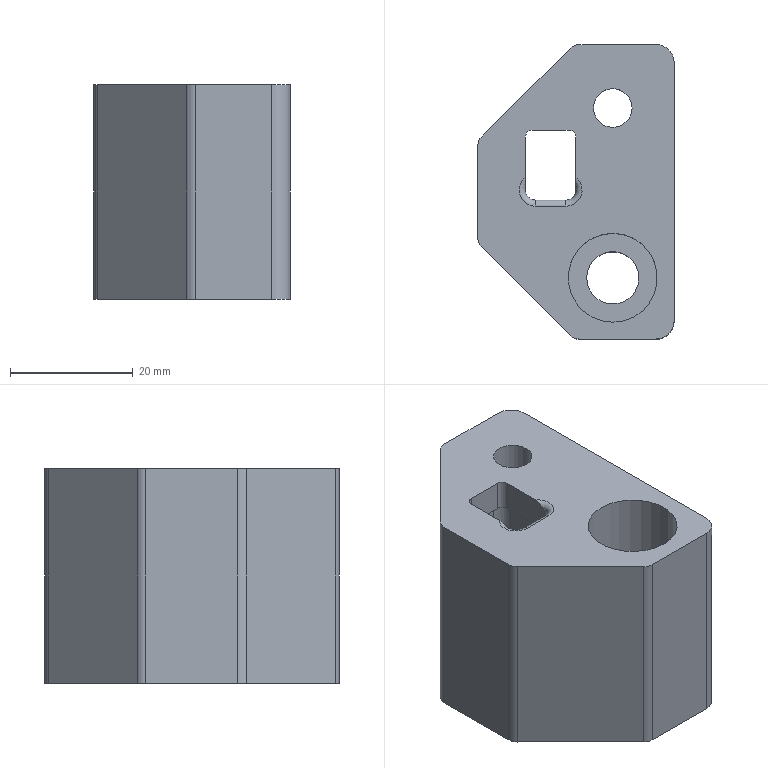Part | NX | features DIE-14 2 | 1 solid | 39 faces | box 32 x 48 x 35 mm | volume 36038 mm3 | cylinder 19 | plane 18 | torus 2 | commonest cylinder face diameters 4 x6 2.24 x2 3.24 x2 5 x2 6 x2 2 x1
STEP:
#1=CARTESIAN_POINT('',(2411.699,-953.548,823.716));
#2=VERTEX_POINT('',#1);
#3=CARTESIAN_POINT('',(2411.699,-911.548,823.716));
#4=VERTEX_POINT('',#3);
#5=CARTESIAN_POINT('',(2411.699,-928.548,823.716));
#6=DIRECTION('',(0.,1.,0.));
#7=VECTOR('',#6,1000.);
#8=LINE('',#5,#7);
#9=EDGE_CURVE('',#2,#4,#8,.T.);
#10=ORIENTED_EDGE('',*,*,#9,.T.);
#11=CARTESIAN_POINT('',(2411.699,-911.548,858.716));
#12=VERTEX_POINT('',#11);
#13=CARTESIAN_POINT('',(2411.699,-911.548,858.716));
#14=DIRECTION('',(0.,0.,1.));
#15=VECTOR('',#14,1000.);
#16=LINE('',#13,#15);
#17=EDGE_CURVE('',#4,#12,#16,.T.);
#18=ORIENTED_EDGE('',*,*,#17,.T.);
#19=CARTESIAN_POINT('',(2411.699,-953.548,858.716));
#20=VERTEX_POINT('',#19);
#21=CARTESIAN_POINT('',(2411.699,-928.548,858.716));
#22=DIRECTION('',(0.,-1.,0.));
#23=VECTOR('',#22,1000.);
#24=LINE('',#21,#23);
#25=EDGE_CURVE('',#12,#20,#24,.T.);
#26=ORIENTED_EDGE('',*,*,#25,.T.);
#27=CARTESIAN_POINT('',(2411.699,-953.548,858.716));
#28=DIRECTION('',(0.,0.,1.));
#29=VECTOR('',#28,1000.);
#30=LINE('',#27,#29);
#31=EDGE_CURVE('',#20,#2,#30,.F.);
#32=ORIENTED_EDGE('',*,*,#31,.T.);
#33=EDGE_LOOP('',(#10,#18,#26,#32));
#34=FACE_BOUND('',#33,.T.);
#35=CARTESIAN_POINT('',(2411.699,-928.548,858.716));
#36=DIRECTION('',(1.,0.,0.));
#37=DIRECTION('',(0.,0.,1.));
#38=AXIS2_PLACEMENT_3D('',#35,#36,#37);
#39=PLANE('',#38);
#40=ADVANCED_FACE('',(#34),#39,.T.);
#41=CARTESIAN_POINT('',(2396.185,-908.548,858.716));
#42=VERTEX_POINT('',#41);
#43=CARTESIAN_POINT('',(2408.699,-908.548,858.716));
#44=VERTEX_POINT('',#43);
#45=CARTESIAN_POINT('',(2401.699,-908.548,858.716));
#46=DIRECTION('',(1.,0.,0.));
#47=VECTOR('',#46,1000.);
#48=LINE('',#45,#47);
#49=EDGE_CURVE('',#42,#44,#48,.T.);
#50=ORIENTED_EDGE('',*,*,#49,.T.);
#51=CARTESIAN_POINT('',(2408.699,-908.548,823.716));
#52=VERTEX_POINT('',#51);
#53=CARTESIAN_POINT('',(2408.699,-908.548,858.716));
#54=DIRECTION('',(0.,0.,1.));
#55=VECTOR('',#54,1000.);
#56=LINE('',#53,#55);
#57=EDGE_CURVE('',#44,#52,#56,.F.);
#58=ORIENTED_EDGE('',*,*,#57,.T.);
#59=CARTESIAN_POINT('',(2396.185,-908.548,823.716));
#60=VERTEX_POINT('',#59);
#61=CARTESIAN_POINT('',(2401.699,-908.548,823.716));
#62=DIRECTION('',(-1.,0.,0.));
#63=VECTOR('',#62,1000.);
#64=LINE('',#61,#63);
#65=EDGE_CURVE('',#52,#60,#64,.T.);
#66=ORIENTED_EDGE('',*,*,#65,.T.);
#67=CARTESIAN_POINT('',(2396.185,-908.548,858.716));
#68=DIRECTION('',(0.,0.,-1.));
#69=VECTOR('',#68,1000.);
#70=LINE('',#67,#69);
#71=EDGE_CURVE('',#60,#42,#70,.F.);
#72=ORIENTED_EDGE('',*,*,#71,.T.);
#73=EDGE_LOOP('',(#50,#58,#66,#72));
#74=FACE_BOUND('',#73,.T.);
#75=CARTESIAN_POINT('',(2401.699,-908.548,858.716));
#76=DIRECTION('',(0.,1.,0.));
#77=DIRECTION('',(0.,0.,-1.));
#78=AXIS2_PLACEMENT_3D('',#75,#76,#77);
#79=PLANE('',#78);
#80=ADVANCED_FACE('',(#74),#79,.T.);
#81=CARTESIAN_POINT('',(2379.699,-940.012,858.716));
#82=VERTEX_POINT('',#81);
#83=CARTESIAN_POINT('',(2379.699,-925.033,858.716));
#84=VERTEX_POINT('',#83);
#85=CARTESIAN_POINT('',(2379.699,-928.548,858.716));
#86=DIRECTION('',(0.,1.,0.));
#87=VECTOR('',#86,1000.);
#88=LINE('',#85,#87);
#89=EDGE_CURVE('',#82,#84,#88,.T.);
#90=ORIENTED_EDGE('',*,*,#89,.T.);
#91=CARTESIAN_POINT('',(2379.699,-925.033,823.716));
#92=VERTEX_POINT('',#91);
#93=CARTESIAN_POINT('',(2379.699,-925.033,858.716));
#94=DIRECTION('',(0.,0.,1.));
#95=VECTOR('',#94,1000.);
#96=LINE('',#93,#95);
#97=EDGE_CURVE('',#84,#92,#96,.F.);
#98=ORIENTED_EDGE('',*,*,#97,.T.);
#99=CARTESIAN_POINT('',(2379.699,-940.012,823.716));
#100=VERTEX_POINT('',#99);
#101=CARTESIAN_POINT('',(2379.699,-928.548,823.716));
#102=DIRECTION('',(0.,-1.,0.));
#103=VECTOR('',#102,1000.);
#104=LINE('',#101,#103);
#105=EDGE_CURVE('',#92,#100,#104,.T.);
#106=ORIENTED_EDGE('',*,*,#105,.T.);
#107=CARTESIAN_POINT('',(2379.699,-940.012,858.716));
#108=DIRECTION('',(0.,0.,-1.));
#109=VECTOR('',#108,1000.);
#110=LINE('',#107,#109);
#111=EDGE_CURVE('',#100,#82,#110,.F.);
#112=ORIENTED_EDGE('',*,*,#111,.T.);
#113=EDGE_LOOP('',(#90,#98,#106,#112));
#114=FACE_BOUND('',#113,.T.);
#115=CARTESIAN_POINT('',(2379.699,-928.548,858.716));
#116=DIRECTION('',(-1.,0.,0.));
#117=DIRECTION('',(0.,0.,-1.));
#118=AXIS2_PLACEMENT_3D('',#115,#116,#117);
#119=PLANE('',#118);
#120=ADVANCED_FACE('',(#114),#119,.T.);
#121=CARTESIAN_POINT('',(2396.235,-956.548,823.716));
#122=VERTEX_POINT('',#121);
#123=CARTESIAN_POINT('',(2408.699,-956.548,823.716));
#124=VERTEX_POINT('',#123);
#125=CARTESIAN_POINT('',(2401.699,-956.548,823.716));
#126=DIRECTION('',(1.,0.,0.));
#127=VECTOR('',#126,1000.);
#128=LINE('',#125,#127);
#129=EDGE_CURVE('',#122,#124,#128,.T.);
#130=ORIENTED_EDGE('',*,*,#129,.T.);
#131=CARTESIAN_POINT('',(2408.699,-956.548,858.716));
#132=VERTEX_POINT('',#131);
#133=CARTESIAN_POINT('',(2408.699,-956.548,858.716));
#134=DIRECTION('',(0.,0.,1.));
#135=VECTOR('',#134,1000.);
#136=LINE('',#133,#135);
#137=EDGE_CURVE('',#124,#132,#136,.T.);
#138=ORIENTED_EDGE('',*,*,#137,.T.);
#139=CARTESIAN_POINT('',(2396.235,-956.548,858.716));
#140=VERTEX_POINT('',#139);
#141=CARTESIAN_POINT('',(2401.699,-956.548,858.716));
#142=DIRECTION('',(-1.,0.,0.));
#143=VECTOR('',#142,1000.);
#144=LINE('',#141,#143);
#145=EDGE_CURVE('',#132,#140,#144,.T.);
#146=ORIENTED_EDGE('',*,*,#145,.T.);
#147=CARTESIAN_POINT('',(2396.235,-956.548,858.716));
#148=DIRECTION('',(0.,0.,1.));
#149=VECTOR('',#148,1000.);
#150=LINE('',#147,#149);
#151=EDGE_CURVE('',#140,#122,#150,.F.);
#152=ORIENTED_EDGE('',*,*,#151,.T.);
#153=EDGE_LOOP('',(#130,#138,#146,#152));
#154=FACE_BOUND('',#153,.T.);
#155=CARTESIAN_POINT('',(2401.699,-956.548,858.716));
#156=DIRECTION('',(0.,-1.,0.));
#157=DIRECTION('',(0.,0.,1.));
#158=AXIS2_PLACEMENT_3D('',#155,#156,#157);
#159=PLANE('',#158);
#160=ADVANCED_FACE('',(#154),#159,.T.);
#161=CARTESIAN_POINT('',(2401.699,-939.298,847.716));
#162=VERTEX_POINT('',#161);
#163=CARTESIAN_POINT('',(2401.699,-946.548,847.716));
#164=DIRECTION('',(0.,0.,1.));
#165=DIRECTION('',(0.,1.,0.));
#166=AXIS2_PLACEMENT_3D('',#163,#164,#165);
#167=CIRCLE('',#166,7.25);
#168=EDGE_CURVE('',#162,#162,#167,.F.);
#169=ORIENTED_EDGE('',*,*,#168,.T.);
#170=EDGE_LOOP('',(#169));
#171=FACE_BOUND('',#170,.T.);
#172=CARTESIAN_POINT('',(2401.699,-939.298,858.716));
#173=VERTEX_POINT('',#172);
#174=CARTESIAN_POINT('',(2401.699,-946.548,858.716));
#175=DIRECTION('',(0.,0.,-1.));
#176=DIRECTION('',(0.,1.,0.));
#177=AXIS2_PLACEMENT_3D('',#174,#175,#176);
#178=CIRCLE('',#177,7.25);
#179=EDGE_CURVE('',#173,#173,#178,.T.);
#180=ORIENTED_EDGE('',*,*,#179,.F.);
#181=EDGE_LOOP('',(#180));
#182=FACE_BOUND('',#181,.T.);
#183=CARTESIAN_POINT('',(2401.699,-946.548,847.716));
#184=DIRECTION('',(0.,0.,1.));
#185=DIRECTION('',(0.,1.,0.));
#186=AXIS2_PLACEMENT_3D('',#183,#184,#185);
#187=CYLINDRICAL_SURFACE('',#186,7.25);
#188=ADVANCED_FACE('',(#171,#182),#187,.F.);
#189=CARTESIAN_POINT('',(2396.569,-931.392,853.716));
#190=VERTEX_POINT('',#189);
#191=CARTESIAN_POINT('',(2394.069,-933.892,853.716));
#192=VERTEX_POINT('',#191);
#193=CARTESIAN_POINT('',(2394.069,-931.392,853.716));
#194=DIRECTION('',(0.,0.,1.));
#195=DIRECTION('',(1.,0.,0.));
#196=AXIS2_PLACEMENT_3D('',#193,#194,#195);
#197=CIRCLE('',#196,2.5);
#198=EDGE_CURVE('',#190,#192,#197,.F.);
#199=ORIENTED_EDGE('',*,*,#198,.F.);
#200=CARTESIAN_POINT('',(2396.569,-931.392,823.716));
#201=VERTEX_POINT('',#200);
#202=CARTESIAN_POINT('',(2396.569,-931.392,940.716));
#203=DIRECTION('',(0.,0.,1.));
#204=VECTOR('',#203,1000.);
#205=LINE('',#202,#204);
#206=EDGE_CURVE('',#201,#190,#205,.T.);
#207=ORIENTED_EDGE('',*,*,#206,.F.);
#208=CARTESIAN_POINT('',(2394.069,-933.892,823.716));
#209=VERTEX_POINT('',#208);
#210=CARTESIAN_POINT('',(2394.069,-931.392,823.716));
#211=DIRECTION('',(0.,0.,-1.));
#212=DIRECTION('',(-1.,0.,0.));
#213=AXIS2_PLACEMENT_3D('',#210,#211,#212);
#214=CIRCLE('',#213,2.5);
#215=EDGE_CURVE('',#209,#201,#214,.F.);
#216=ORIENTED_EDGE('',*,*,#215,.F.);
#217=CARTESIAN_POINT('',(2394.069,-933.892,940.716));
#218=DIRECTION('',(0.,0.,1.));
#219=VECTOR('',#218,1000.);
#220=LINE('',#217,#219);
#221=EDGE_CURVE('',#192,#209,#220,.F.);
#222=ORIENTED_EDGE('',*,*,#221,.F.);
#223=EDGE_LOOP('',(#199,#207,#216,#222));
#224=FACE_BOUND('',#223,.T.);
#225=CARTESIAN_POINT('',(2394.069,-931.392,940.716));
#226=DIRECTION('',(0.,0.,-1.));
#227=DIRECTION('',(-1.,0.,0.));
#228=AXIS2_PLACEMENT_3D('',#225,#226,#227);
#229=CYLINDRICAL_SURFACE('',#228,2.5);
#230=ADVANCED_FACE('',(#224),#229,.F.);
#231=CARTESIAN_POINT('',(2386.569,-923.622,853.716));
#232=VERTEX_POINT('',#231);
#233=CARTESIAN_POINT('',(2386.569,-923.622,823.716));
#234=VERTEX_POINT('',#233);
#235=CARTESIAN_POINT('',(2386.569,-923.622,940.716));
#236=DIRECTION('',(0.,0.,-1.));
#237=VECTOR('',#236,1000.);
#238=LINE('',#235,#237);
#239=EDGE_CURVE('',#232,#234,#238,.T.);
#240=ORIENTED_EDGE('',*,*,#239,.F.);
#241=CARTESIAN_POINT('',(2386.569,-931.392,853.716));
#242=VERTEX_POINT('',#241);
#243=CARTESIAN_POINT('',(2386.569,-925.122,853.716));
#244=DIRECTION('',(0.,-1.,0.));
#245=VECTOR('',#244,1000.);
#246=LINE('',#243,#245);
#247=EDGE_CURVE('',#232,#242,#246,.T.);
#248=ORIENTED_EDGE('',*,*,#247,.T.);
#249=CARTESIAN_POINT('',(2386.569,-931.392,823.716));
#250=VERTEX_POINT('',#249);
#251=CARTESIAN_POINT('',(2386.569,-931.392,940.716));
#252=DIRECTION('',(0.,0.,1.));
#253=VECTOR('',#252,1000.);
#254=LINE('',#251,#253);
#255=EDGE_CURVE('',#242,#250,#254,.F.);
#256=ORIENTED_EDGE('',*,*,#255,.T.);
#257=CARTESIAN_POINT('',(2386.569,-925.122,823.716));
#258=DIRECTION('',(0.,1.,0.));
#259=VECTOR('',#258,1000.);
#260=LINE('',#257,#259);
#261=EDGE_CURVE('',#250,#234,#260,.T.);
#262=ORIENTED_EDGE('',*,*,#261,.T.);
#263=EDGE_LOOP('',(#240,#248,#256,#262));
#264=FACE_BOUND('',#263,.T.);
#265=CARTESIAN_POINT('',(2386.569,-925.122,940.716));
#266=DIRECTION('',(1.,0.,0.));
#267=DIRECTION('',(0.,0.,1.));
#268=AXIS2_PLACEMENT_3D('',#265,#266,#267);
#269=PLANE('',#268);
#270=ADVANCED_FACE('',(#264),#269,.T.);
#271=CARTESIAN_POINT('',(2389.069,-933.892,853.716));
#272=VERTEX_POINT('',#271);
#273=CARTESIAN_POINT('',(2389.069,-933.892,857.716));
#274=VERTEX_POINT('',#273);
#275=CARTESIAN_POINT('',(2389.069,-933.892,940.716));
#276=DIRECTION('',(0.,0.,-1.));
#277=VECTOR('',#276,1000.);
#278=LINE('',#275,#277);
#279=EDGE_CURVE('',#272,#274,#278,.F.);
#280=ORIENTED_EDGE('',*,*,#279,.T.);
#281=CARTESIAN_POINT('',(2394.069,-933.892,857.716));
#282=VERTEX_POINT('',#281);
#283=CARTESIAN_POINT('',(2388.419,-933.892,857.716));
#284=DIRECTION('',(-1.,0.,0.));
#285=VECTOR('',#284,1000.);
#286=LINE('',#283,#285);
#287=EDGE_CURVE('',#274,#282,#286,.F.);
#288=ORIENTED_EDGE('',*,*,#287,.T.);
#289=CARTESIAN_POINT('',(2394.069,-933.892,940.716));
#290=DIRECTION('',(0.,0.,-1.));
#291=VECTOR('',#290,1000.);
#292=LINE('',#289,#291);
#293=EDGE_CURVE('',#282,#192,#292,.T.);
#294=ORIENTED_EDGE('',*,*,#293,.T.);
#295=ORIENTED_EDGE('',*,*,#221,.T.);
#296=CARTESIAN_POINT('',(2389.069,-933.892,823.716));
#297=VERTEX_POINT('',#296);
#298=CARTESIAN_POINT('',(2388.419,-933.892,823.716));
#299=DIRECTION('',(-1.,0.,0.));
#300=VECTOR('',#299,1000.);
#301=LINE('',#298,#300);
#302=EDGE_CURVE('',#209,#297,#301,.T.);
#303=ORIENTED_EDGE('',*,*,#302,.T.);
#304=CARTESIAN_POINT('',(2389.069,-933.892,940.716));
#305=DIRECTION('',(0.,0.,1.));
#306=VECTOR('',#305,1000.);
#307=LINE('',#304,#306);
#308=EDGE_CURVE('',#297,#272,#307,.T.);
#309=ORIENTED_EDGE('',*,*,#308,.T.);
#310=EDGE_LOOP('',(#280,#288,#294,#295,#303,#309));
#311=FACE_BOUND('',#310,.T.);
#312=CARTESIAN_POINT('',(2388.419,-933.892,940.716));
#313=DIRECTION('',(0.,1.,0.));
#314=DIRECTION('',(0.,0.,-1.));
#315=AXIS2_PLACEMENT_3D('',#312,#313,#314);
#316=PLANE('',#315);
#317=ADVANCED_FACE('',(#311),#316,.T.);
#318=CARTESIAN_POINT('',(2394.569,-921.622,853.716));
#319=VERTEX_POINT('',#318);
#320=CARTESIAN_POINT('',(2394.569,-921.622,823.716));
#321=VERTEX_POINT('',#320);
#322=CARTESIAN_POINT('',(2394.569,-921.622,940.716));
#323=DIRECTION('',(0.,0.,-1.));
#324=VECTOR('',#323,1000.);
#325=LINE('',#322,#324);
#326=EDGE_CURVE('',#319,#321,#325,.T.);
#327=ORIENTED_EDGE('',*,*,#326,.F.);
#328=CARTESIAN_POINT('',(2388.569,-921.622,853.716));
#329=VERTEX_POINT('',#328);
#330=CARTESIAN_POINT('',(2393.069,-921.622,853.716));
#331=DIRECTION('',(-1.,0.,0.));
#332=VECTOR('',#331,1000.);
#333=LINE('',#330,#332);
#334=EDGE_CURVE('',#319,#329,#333,.T.);
#335=ORIENTED_EDGE('',*,*,#334,.T.);
#336=CARTESIAN_POINT('',(2388.569,-921.622,823.716));
#337=VERTEX_POINT('',#336);
#338=CARTESIAN_POINT('',(2388.569,-921.622,940.716));
#339=DIRECTION('',(0.,0.,-1.));
#340=VECTOR('',#339,1000.);
#341=LINE('',#338,#340);
#342=EDGE_CURVE('',#337,#329,#341,.F.);
#343=ORIENTED_EDGE('',*,*,#342,.F.);
#344=CARTESIAN_POINT('',(2401.699,-921.622,823.716));
#345=DIRECTION('',(-1.,0.,0.));
#346=VECTOR('',#345,1000.);
#347=LINE('',#344,#346);
#348=EDGE_CURVE('',#321,#337,#347,.T.);
#349=ORIENTED_EDGE('',*,*,#348,.F.);
#350=EDGE_LOOP('',(#327,#335,#343,#349));
#351=FACE_BOUND('',#350,.T.);
#352=CARTESIAN_POINT('',(2393.069,-921.622,940.716));
#353=DIRECTION('',(0.,-1.,0.));
#354=DIRECTION('',(0.,0.,1.));
#355=AXIS2_PLACEMENT_3D('',#352,#353,#354);
#356=PLANE('',#355);
#357=ADVANCED_FACE('',(#351),#356,.T.);
#358=CARTESIAN_POINT('',(2389.069,-931.392,853.716));
#359=DIRECTION('',(0.,0.,1.));
#360=DIRECTION('',(1.,0.,0.));
#361=AXIS2_PLACEMENT_3D('',#358,#359,#360);
#362=CIRCLE('',#361,2.5);
#363=EDGE_CURVE('',#272,#242,#362,.F.);
#364=ORIENTED_EDGE('',*,*,#363,.F.);
#365=ORIENTED_EDGE('',*,*,#308,.F.);
#366=CARTESIAN_POINT('',(2389.069,-931.392,823.716));
#367=DIRECTION('',(0.,0.,-1.));
#368=DIRECTION('',(-1.,0.,0.));
#369=AXIS2_PLACEMENT_3D('',#366,#367,#368);
#370=CIRCLE('',#369,2.5);
#371=EDGE_CURVE('',#250,#297,#370,.F.);
#372=ORIENTED_EDGE('',*,*,#371,.F.);
#373=ORIENTED_EDGE('',*,*,#255,.F.);
#374=EDGE_LOOP('',(#364,#365,#372,#373));
#375=FACE_BOUND('',#374,.T.);
#376=CARTESIAN_POINT('',(2389.069,-931.392,940.716));
#377=DIRECTION('',(0.,0.,-1.));
#378=DIRECTION('',(-1.,0.,0.));
#379=AXIS2_PLACEMENT_3D('',#376,#377,#378);
#380=CYLINDRICAL_SURFACE('',#379,2.5);
#381=ADVANCED_FACE('',(#375),#380,.F.);
#382=ORIENTED_EDGE('',*,*,#206,.T.);
#383=CARTESIAN_POINT('',(2396.569,-923.622,853.716));
#384=VERTEX_POINT('',#383);
#385=CARTESIAN_POINT('',(2396.569,-932.772,853.716));
#386=DIRECTION('',(0.,1.,0.));
#387=VECTOR('',#386,1000.);
#388=LINE('',#385,#387);
#389=EDGE_CURVE('',#190,#384,#388,.T.);
#390=ORIENTED_EDGE('',*,*,#389,.T.);
#391=CARTESIAN_POINT('',(2396.569,-923.622,823.716));
#392=VERTEX_POINT('',#391);
#393=CARTESIAN_POINT('',(2396.569,-923.622,940.716));
#394=DIRECTION('',(0.,0.,-1.));
#395=VECTOR('',#394,1000.);
#396=LINE('',#393,#395);
#397=EDGE_CURVE('',#392,#384,#396,.F.);
#398=ORIENTED_EDGE('',*,*,#397,.F.);
#399=CARTESIAN_POINT('',(2396.569,-932.772,823.716));
#400=DIRECTION('',(0.,-1.,0.));
#401=VECTOR('',#400,1000.);
#402=LINE('',#399,#401);
#403=EDGE_CURVE('',#392,#201,#402,.T.);
#404=ORIENTED_EDGE('',*,*,#403,.T.);
#405=EDGE_LOOP('',(#382,#390,#398,#404));
#406=FACE_BOUND('',#405,.T.);
#407=CARTESIAN_POINT('',(2396.569,-932.772,940.716));
#408=DIRECTION('',(-1.,0.,0.));
#409=DIRECTION('',(0.,0.,-1.));
#410=AXIS2_PLACEMENT_3D('',#407,#408,#409);
#411=PLANE('',#410);
#412=ADVANCED_FACE('',(#406),#411,.T.);
#413=CARTESIAN_POINT('',(2388.569,-923.622,853.716));
#414=DIRECTION('',(0.,0.,1.));
#415=DIRECTION('',(1.,0.,0.));
#416=AXIS2_PLACEMENT_3D('',#413,#414,#415);
#417=CIRCLE('',#416,2.);
#418=EDGE_CURVE('',#232,#329,#417,.F.);
#419=ORIENTED_EDGE('',*,*,#418,.F.);
#420=ORIENTED_EDGE('',*,*,#239,.T.);
#421=CARTESIAN_POINT('',(2388.569,-923.622,823.716));
#422=DIRECTION('',(0.,0.,-1.));
#423=DIRECTION('',(-1.,0.,0.));
#424=AXIS2_PLACEMENT_3D('',#421,#422,#423);
#425=CIRCLE('',#424,2.);
#426=EDGE_CURVE('',#234,#337,#425,.T.);
#427=ORIENTED_EDGE('',*,*,#426,.T.);
#428=ORIENTED_EDGE('',*,*,#342,.T.);
#429=EDGE_LOOP('',(#419,#420,#427,#428));
#430=FACE_BOUND('',#429,.T.);
#431=CARTESIAN_POINT('',(2388.569,-923.622,940.716));
#432=DIRECTION('',(0.,0.,-1.));
#433=DIRECTION('',(1.,0.,0.));
#434=AXIS2_PLACEMENT_3D('',#431,#432,#433);
#435=CYLINDRICAL_SURFACE('',#434,2.);
#436=ADVANCED_FACE('',(#430),#435,.F.);
#437=CARTESIAN_POINT('',(2394.569,-923.622,853.716));
#438=DIRECTION('',(0.,0.,1.));
#439=DIRECTION('',(1.,0.,0.));
#440=AXIS2_PLACEMENT_3D('',#437,#438,#439);
#441=CIRCLE('',#440,2.);
#442=EDGE_CURVE('',#319,#384,#441,.F.);
#443=ORIENTED_EDGE('',*,*,#442,.F.);
#444=ORIENTED_EDGE('',*,*,#326,.T.);
#445=CARTESIAN_POINT('',(2394.569,-923.622,823.716));
#446=DIRECTION('',(0.,0.,-1.));
#447=DIRECTION('',(-1.,0.,0.));
#448=AXIS2_PLACEMENT_3D('',#445,#446,#447);
#449=CIRCLE('',#448,2.);
#450=EDGE_CURVE('',#392,#321,#449,.F.);
#451=ORIENTED_EDGE('',*,*,#450,.F.);
#452=ORIENTED_EDGE('',*,*,#397,.T.);
#453=EDGE_LOOP('',(#443,#444,#451,#452));
#454=FACE_BOUND('',#453,.T.);
#455=CARTESIAN_POINT('',(2394.569,-923.622,940.716));
#456=DIRECTION('',(0.,0.,-1.));
#457=DIRECTION('',(1.,0.,0.));
#458=AXIS2_PLACEMENT_3D('',#455,#456,#457);
#459=CYLINDRICAL_SURFACE('',#458,2.);
#460=ADVANCED_FACE('',(#454),#459,.F.);
#461=CARTESIAN_POINT('',(2397.554,-918.898,823.716));
#462=VERTEX_POINT('',#461);
#463=CARTESIAN_POINT('',(2401.699,-918.898,823.716));
#464=DIRECTION('',(0.,0.,1.));
#465=DIRECTION('',(-1.,0.,0.));
#466=AXIS2_PLACEMENT_3D('',#463,#464,#465);
#467=CIRCLE('',#466,4.145);
#468=EDGE_CURVE('',#462,#462,#467,.F.);
#469=ORIENTED_EDGE('',*,*,#468,.F.);
#470=EDGE_LOOP('',(#469));
#471=FACE_BOUND('',#470,.T.);
#472=CARTESIAN_POINT('',(2405.952,-946.548,823.716));
#473=VERTEX_POINT('',#472);
#474=CARTESIAN_POINT('',(2401.699,-946.548,823.716));
#475=DIRECTION('',(0.,0.,-1.));
#476=DIRECTION('',(1.,0.,0.));
#477=AXIS2_PLACEMENT_3D('',#474,#475,#476);
#478=CIRCLE('',#477,4.253);
#479=EDGE_CURVE('',#473,#473,#478,.T.);
#480=ORIENTED_EDGE('',*,*,#479,.F.);
#481=EDGE_LOOP('',(#480));
#482=FACE_BOUND('',#481,.T.);
#483=ORIENTED_EDGE('',*,*,#65,.F.);
#484=CARTESIAN_POINT('',(2408.699,-911.548,823.716));
#485=DIRECTION('',(0.,0.,-1.));
#486=DIRECTION('',(-1.,0.,0.));
#487=AXIS2_PLACEMENT_3D('',#484,#485,#486);
#488=CIRCLE('',#487,3.);
#489=EDGE_CURVE('',#52,#4,#488,.T.);
#490=ORIENTED_EDGE('',*,*,#489,.T.);
#491=ORIENTED_EDGE('',*,*,#9,.F.);
#492=CARTESIAN_POINT('',(2408.699,-953.548,823.716));
#493=DIRECTION('',(0.,0.,-1.));
#494=DIRECTION('',(-1.,0.,0.));
#495=AXIS2_PLACEMENT_3D('',#492,#493,#494);
#496=CIRCLE('',#495,3.);
#497=EDGE_CURVE('',#2,#124,#496,.T.);
#498=ORIENTED_EDGE('',*,*,#497,.T.);
#499=ORIENTED_EDGE('',*,*,#129,.F.);
#500=CARTESIAN_POINT('',(2394.821,-955.962,823.716));
#501=VERTEX_POINT('',#500);
#502=CARTESIAN_POINT('',(2396.235,-954.548,823.716));
#503=DIRECTION('',(0.,0.,-1.));
#504=DIRECTION('',(-1.,0.,0.));
#505=AXIS2_PLACEMENT_3D('',#502,#503,#504);
#506=CIRCLE('',#505,2.);
#507=EDGE_CURVE('',#122,#501,#506,.T.);
#508=ORIENTED_EDGE('',*,*,#507,.T.);
#509=CARTESIAN_POINT('',(2380.285,-941.426,823.716));
#510=VERTEX_POINT('',#509);
#511=CARTESIAN_POINT('',(2384.553,-945.694,823.716));
#512=DIRECTION('',(0.7071,-0.7071,0.));
#513=VECTOR('',#512,1000.);
#514=LINE('',#511,#513);
#515=EDGE_CURVE('',#501,#510,#514,.F.);
#516=ORIENTED_EDGE('',*,*,#515,.T.);
#517=CARTESIAN_POINT('',(2381.699,-940.012,823.716));
#518=DIRECTION('',(0.,0.,-1.));
#519=DIRECTION('',(-1.,0.,0.));
#520=AXIS2_PLACEMENT_3D('',#517,#518,#519);
#521=CIRCLE('',#520,2.);
#522=EDGE_CURVE('',#510,#100,#521,.T.);
#523=ORIENTED_EDGE('',*,*,#522,.T.);
#524=ORIENTED_EDGE('',*,*,#105,.F.);
#525=CARTESIAN_POINT('',(2380.285,-923.619,823.716));
#526=VERTEX_POINT('',#525);
#527=CARTESIAN_POINT('',(2381.699,-925.033,823.716));
#528=DIRECTION('',(0.,0.,-1.));
#529=DIRECTION('',(-1.,0.,0.));
#530=AXIS2_PLACEMENT_3D('',#527,#528,#529);
#531=CIRCLE('',#530,2.);
#532=EDGE_CURVE('',#92,#526,#531,.T.);
#533=ORIENTED_EDGE('',*,*,#532,.T.);
#534=CARTESIAN_POINT('',(2394.77,-909.133,823.716));
#535=VERTEX_POINT('',#534);
#536=CARTESIAN_POINT('',(2388.528,-915.376,823.716));
#537=DIRECTION('',(-0.7071,-0.7071,0.));
#538=VECTOR('',#537,1000.);
#539=LINE('',#536,#538);
#540=EDGE_CURVE('',#526,#535,#539,.F.);
#541=ORIENTED_EDGE('',*,*,#540,.T.);
#542=CARTESIAN_POINT('',(2396.185,-910.548,823.716));
#543=DIRECTION('',(0.,0.,-1.));
#544=DIRECTION('',(-1.,0.,0.));
#545=AXIS2_PLACEMENT_3D('',#542,#543,#544);
#546=CIRCLE('',#545,2.);
#547=EDGE_CURVE('',#535,#60,#546,.T.);
#548=ORIENTED_EDGE('',*,*,#547,.T.);
#549=EDGE_LOOP('',(#483,#490,#491,#498,#499,#508,#516,#523,#524,#533,#541,#548));
#550=FACE_BOUND('',#549,.T.);
#551=ORIENTED_EDGE('',*,*,#261,.F.);
#552=ORIENTED_EDGE('',*,*,#371,.T.);
#553=ORIENTED_EDGE('',*,*,#302,.F.);
#554=ORIENTED_EDGE('',*,*,#215,.T.);
#555=ORIENTED_EDGE('',*,*,#403,.F.);
#556=ORIENTED_EDGE('',*,*,#450,.T.);
#557=ORIENTED_EDGE('',*,*,#348,.T.);
#558=ORIENTED_EDGE('',*,*,#426,.F.);
#559=EDGE_LOOP('',(#551,#552,#553,#554,#555,#556,#557,#558));
#560=FACE_BOUND('',#559,.T.);
#561=CARTESIAN_POINT('',(2401.699,-928.548,823.716));
#562=DIRECTION('',(0.,0.,-1.));
#563=DIRECTION('',(0.,-1.,0.));
#564=AXIS2_PLACEMENT_3D('',#561,#562,#563);
#565=PLANE('',#564);
#566=ADVANCED_FACE('',(#471,#482,#550,#560),#565,.T.);
#567=ORIENTED_EDGE('',*,*,#468,.T.);
#568=EDGE_LOOP('',(#567));
#569=FACE_BOUND('',#568,.T.);
#570=CARTESIAN_POINT('',(2405.844,-918.898,853.716));
#571=VERTEX_POINT('',#570);
#572=CARTESIAN_POINT('',(2401.699,-918.898,853.716));
#573=DIRECTION('',(0.,0.,-1.));
#574=DIRECTION('',(1.,0.,0.));
#575=AXIS2_PLACEMENT_3D('',#572,#573,#574);
#576=CIRCLE('',#575,4.145);
#577=EDGE_CURVE('',#571,#571,#576,.T.);
#578=ORIENTED_EDGE('',*,*,#577,.F.);
#579=EDGE_LOOP('',(#578));
#580=FACE_BOUND('',#579,.T.);
#581=CARTESIAN_POINT('',(2401.699,-918.898,858.716));
#582=DIRECTION('',(0.,0.,-1.));
#583=DIRECTION('',(1.,0.,0.));
#584=AXIS2_PLACEMENT_3D('',#581,#582,#583);
#585=CYLINDRICAL_SURFACE('',#584,4.145);
#586=ADVANCED_FACE('',(#569,#580),#585,.F.);
#587=CARTESIAN_POINT('',(2405.952,-946.548,847.716));
#588=VERTEX_POINT('',#587);
#589=CARTESIAN_POINT('',(2401.699,-946.548,847.716));
#590=DIRECTION('',(0.,0.,-1.));
#591=DIRECTION('',(1.,0.,0.));
#592=AXIS2_PLACEMENT_3D('',#589,#590,#591);
#593=CIRCLE('',#592,4.253);
#594=EDGE_CURVE('',#588,#588,#593,.T.);
#595=ORIENTED_EDGE('',*,*,#594,.T.);
#596=EDGE_LOOP('',(#595));
#597=FACE_BOUND('',#596,.T.);
#598=ORIENTED_EDGE('',*,*,#168,.F.);
#599=EDGE_LOOP('',(#598));
#600=FACE_BOUND('',#599,.T.);
#601=CARTESIAN_POINT('',(2401.699,-946.548,847.716));
#602=DIRECTION('',(0.,0.,-1.));
#603=DIRECTION('',(1.,0.,0.));
#604=AXIS2_PLACEMENT_3D('',#601,#602,#603);
#605=PLANE('',#604);
#606=ADVANCED_FACE('',(#597,#600),#605,.F.);
#607=ORIENTED_EDGE('',*,*,#479,.T.);
#608=EDGE_LOOP('',(#607));
#609=FACE_BOUND('',#608,.T.);
#610=ORIENTED_EDGE('',*,*,#594,.F.);
#611=EDGE_LOOP('',(#610));
#612=FACE_BOUND('',#611,.T.);
#613=CARTESIAN_POINT('',(2401.699,-946.548,822.716));
#614=DIRECTION('',(0.,0.,1.));
#615=DIRECTION('',(0.,1.,0.));
#616=AXIS2_PLACEMENT_3D('',#613,#614,#615);
#617=CYLINDRICAL_SURFACE('',#616,4.253);
#618=ADVANCED_FACE('',(#609,#612),#617,.F.);
#619=CARTESIAN_POINT('',(2404.844,-918.898,853.716));
#620=VERTEX_POINT('',#619);
#621=CARTESIAN_POINT('',(2401.699,-918.898,853.716));
#622=DIRECTION('',(0.,0.,1.));
#623=DIRECTION('',(1.,0.,0.));
#624=AXIS2_PLACEMENT_3D('',#621,#622,#623);
#625=CIRCLE('',#624,3.145);
#626=EDGE_CURVE('',#620,#620,#625,.T.);
#627=ORIENTED_EDGE('',*,*,#626,.T.);
#628=EDGE_LOOP('',(#627));
#629=FACE_BOUND('',#628,.T.);
#630=ORIENTED_EDGE('',*,*,#577,.T.);
#631=EDGE_LOOP('',(#630));
#632=FACE_BOUND('',#631,.T.);
#633=CARTESIAN_POINT('',(2401.699,-927.548,853.716));
#634=DIRECTION('',(0.,0.,1.));
#635=DIRECTION('',(1.,0.,0.));
#636=AXIS2_PLACEMENT_3D('',#633,#634,#635);
#637=PLANE('',#636);
#638=ADVANCED_FACE('',(#629,#632),#637,.F.);
#639=CARTESIAN_POINT('',(2395.689,-923.622,858.716));
#640=VERTEX_POINT('',#639);
#641=CARTESIAN_POINT('',(2395.689,-930.213,858.716));
#642=VERTEX_POINT('',#641);
#643=CARTESIAN_POINT('',(2395.689,-928.548,858.716));
#644=DIRECTION('',(0.,-1.,0.));
#645=VECTOR('',#644,1000.);
#646=LINE('',#643,#645);
#647=EDGE_CURVE('',#640,#642,#646,.T.);
#648=ORIENTED_EDGE('',*,*,#647,.T.);
#649=CARTESIAN_POINT('',(2394.069,-934.892,858.716));
#650=VERTEX_POINT('',#649);
#651=CARTESIAN_POINT('',(2394.069,-932.272,858.716));
#652=DIRECTION('',(0.,0.,1.));
#653=DIRECTION('',(1.,0.,0.));
#654=AXIS2_PLACEMENT_3D('',#651,#652,#653);
#655=CIRCLE('',#654,2.62);
#656=EDGE_CURVE('',#642,#650,#655,.F.);
#657=ORIENTED_EDGE('',*,*,#656,.T.);
#658=CARTESIAN_POINT('',(2389.069,-934.892,858.716));
#659=VERTEX_POINT('',#658);
#660=CARTESIAN_POINT('',(2401.699,-934.892,858.716));
#661=DIRECTION('',(-1.,0.,0.));
#662=VECTOR('',#661,1000.);
#663=LINE('',#660,#662);
#664=EDGE_CURVE('',#650,#659,#663,.T.);
#665=ORIENTED_EDGE('',*,*,#664,.T.);
#666=CARTESIAN_POINT('',(2387.449,-930.213,858.716));
#667=VERTEX_POINT('',#666);
#668=CARTESIAN_POINT('',(2389.069,-932.272,858.716));
#669=DIRECTION('',(0.,0.,1.));
#670=DIRECTION('',(1.,0.,0.));
#671=AXIS2_PLACEMENT_3D('',#668,#669,#670);
#672=CIRCLE('',#671,2.62);
#673=EDGE_CURVE('',#659,#667,#672,.F.);
#674=ORIENTED_EDGE('',*,*,#673,.T.);
#675=CARTESIAN_POINT('',(2387.449,-923.622,858.716));
#676=VERTEX_POINT('',#675);
#677=CARTESIAN_POINT('',(2387.449,-928.548,858.716));
#678=DIRECTION('',(0.,1.,0.));
#679=VECTOR('',#678,1000.);
#680=LINE('',#677,#679);
#681=EDGE_CURVE('',#667,#676,#680,.T.);
#682=ORIENTED_EDGE('',*,*,#681,.T.);
#683=CARTESIAN_POINT('',(2388.569,-922.502,858.716));
#684=VERTEX_POINT('',#683);
#685=CARTESIAN_POINT('',(2388.569,-923.622,858.716));
#686=DIRECTION('',(0.,0.,1.));
#687=DIRECTION('',(1.,0.,0.));
#688=AXIS2_PLACEMENT_3D('',#685,#686,#687);
#689=CIRCLE('',#688,1.12);
#690=EDGE_CURVE('',#684,#676,#689,.T.);
#691=ORIENTED_EDGE('',*,*,#690,.F.);
#692=CARTESIAN_POINT('',(2394.569,-922.502,858.716));
#693=VERTEX_POINT('',#692);
#694=CARTESIAN_POINT('',(2401.699,-922.502,858.716));
#695=DIRECTION('',(1.,0.,0.));
#696=VECTOR('',#695,1000.);
#697=LINE('',#694,#696);
#698=EDGE_CURVE('',#684,#693,#697,.T.);
#699=ORIENTED_EDGE('',*,*,#698,.T.);
#700=CARTESIAN_POINT('',(2394.569,-923.622,858.716));
#701=DIRECTION('',(0.,0.,1.));
#702=DIRECTION('',(1.,0.,0.));
#703=AXIS2_PLACEMENT_3D('',#700,#701,#702);
#704=CIRCLE('',#703,1.12);
#705=EDGE_CURVE('',#640,#693,#704,.T.);
#706=ORIENTED_EDGE('',*,*,#705,.F.);
#707=EDGE_LOOP('',(#648,#657,#665,#674,#682,#691,#699,#706));
#708=FACE_BOUND('',#707,.T.);
#709=ORIENTED_EDGE('',*,*,#179,.T.);
#710=EDGE_LOOP('',(#709));
#711=FACE_BOUND('',#710,.T.);
#712=CARTESIAN_POINT('',(2404.844,-918.898,858.716));
#713=VERTEX_POINT('',#712);
#714=CARTESIAN_POINT('',(2401.699,-918.898,858.716));
#715=DIRECTION('',(0.,0.,1.));
#716=DIRECTION('',(1.,0.,0.));
#717=AXIS2_PLACEMENT_3D('',#714,#715,#716);
#718=CIRCLE('',#717,3.145);
#719=EDGE_CURVE('',#713,#713,#718,.T.);
#720=ORIENTED_EDGE('',*,*,#719,.F.);
#721=EDGE_LOOP('',(#720));
#722=FACE_BOUND('',#721,.T.);
#723=ORIENTED_EDGE('',*,*,#25,.F.);
#724=CARTESIAN_POINT('',(2408.699,-911.548,858.716));
#725=DIRECTION('',(0.,0.,1.));
#726=DIRECTION('',(1.,0.,0.));
#727=AXIS2_PLACEMENT_3D('',#724,#725,#726);
#728=CIRCLE('',#727,3.);
#729=EDGE_CURVE('',#12,#44,#728,.T.);
#730=ORIENTED_EDGE('',*,*,#729,.T.);
#731=ORIENTED_EDGE('',*,*,#49,.F.);
#732=CARTESIAN_POINT('',(2394.77,-909.133,858.716));
#733=VERTEX_POINT('',#732);
#734=CARTESIAN_POINT('',(2396.185,-910.548,858.716));
#735=DIRECTION('',(0.,0.,1.));
#736=DIRECTION('',(1.,0.,0.));
#737=AXIS2_PLACEMENT_3D('',#734,#735,#736);
#738=CIRCLE('',#737,2.);
#739=EDGE_CURVE('',#42,#733,#738,.T.);
#740=ORIENTED_EDGE('',*,*,#739,.T.);
#741=CARTESIAN_POINT('',(2380.285,-923.619,858.716));
#742=VERTEX_POINT('',#741);
#743=CARTESIAN_POINT('',(2388.528,-915.376,858.716));
#744=DIRECTION('',(0.7071,0.7071,0.));
#745=VECTOR('',#744,1000.);
#746=LINE('',#743,#745);
#747=EDGE_CURVE('',#733,#742,#746,.F.);
#748=ORIENTED_EDGE('',*,*,#747,.T.);
#749=CARTESIAN_POINT('',(2381.699,-925.033,858.716));
#750=DIRECTION('',(0.,0.,1.));
#751=DIRECTION('',(1.,0.,0.));
#752=AXIS2_PLACEMENT_3D('',#749,#750,#751);
#753=CIRCLE('',#752,2.);
#754=EDGE_CURVE('',#742,#84,#753,.T.);
#755=ORIENTED_EDGE('',*,*,#754,.T.);
#756=ORIENTED_EDGE('',*,*,#89,.F.);
#757=CARTESIAN_POINT('',(2380.285,-941.426,858.716));
#758=VERTEX_POINT('',#757);
#759=CARTESIAN_POINT('',(2381.699,-940.012,858.716));
#760=DIRECTION('',(0.,0.,1.));
#761=DIRECTION('',(1.,0.,0.));
#762=AXIS2_PLACEMENT_3D('',#759,#760,#761);
#763=CIRCLE('',#762,2.);
#764=EDGE_CURVE('',#82,#758,#763,.T.);
#765=ORIENTED_EDGE('',*,*,#764,.T.);
#766=CARTESIAN_POINT('',(2394.821,-955.962,858.716));
#767=VERTEX_POINT('',#766);
#768=CARTESIAN_POINT('',(2384.553,-945.694,858.716));
#769=DIRECTION('',(-0.7071,0.7071,0.));
#770=VECTOR('',#769,1000.);
#771=LINE('',#768,#770);
#772=EDGE_CURVE('',#758,#767,#771,.F.);
#773=ORIENTED_EDGE('',*,*,#772,.T.);
#774=CARTESIAN_POINT('',(2396.235,-954.548,858.716));
#775=DIRECTION('',(0.,0.,1.));
#776=DIRECTION('',(1.,0.,0.));
#777=AXIS2_PLACEMENT_3D('',#774,#775,#776);
#778=CIRCLE('',#777,2.);
#779=EDGE_CURVE('',#767,#140,#778,.T.);
#780=ORIENTED_EDGE('',*,*,#779,.T.);
#781=ORIENTED_EDGE('',*,*,#145,.F.);
#782=CARTESIAN_POINT('',(2408.699,-953.548,858.716));
#783=DIRECTION('',(0.,0.,1.));
#784=DIRECTION('',(1.,0.,0.));
#785=AXIS2_PLACEMENT_3D('',#782,#783,#784);
#786=CIRCLE('',#785,3.);
#787=EDGE_CURVE('',#132,#20,#786,.T.);
#788=ORIENTED_EDGE('',*,*,#787,.T.);
#789=EDGE_LOOP('',(#723,#730,#731,#740,#748,#755,#756,#765,#773,#780,#781,#788));
#790=FACE_BOUND('',#789,.T.);
#791=CARTESIAN_POINT('',(2401.699,-928.548,858.716));
#792=DIRECTION('',(0.,0.,1.));
#793=DIRECTION('',(0.,1.,0.));
#794=AXIS2_PLACEMENT_3D('',#791,#792,#793);
#795=PLANE('',#794);
#796=ADVANCED_FACE('',(#708,#711,#722,#790),#795,.T.);
#797=CARTESIAN_POINT('',(2387.449,-932.272,857.716));
#798=VERTEX_POINT('',#797);
#799=CARTESIAN_POINT('',(2387.449,-932.272,853.716));
#800=VERTEX_POINT('',#799);
#801=CARTESIAN_POINT('',(2387.449,-932.272,940.716));
#802=DIRECTION('',(0.,0.,1.));
#803=VECTOR('',#802,1000.);
#804=LINE('',#801,#803);
#805=EDGE_CURVE('',#798,#800,#804,.F.);
#806=ORIENTED_EDGE('',*,*,#805,.F.);
#807=CARTESIAN_POINT('',(2389.069,-932.272,857.716));
#808=DIRECTION('',(0.,0.,1.));
#809=DIRECTION('',(1.,0.,0.));
#810=AXIS2_PLACEMENT_3D('',#807,#808,#809);
#811=CIRCLE('',#810,1.62);
#812=EDGE_CURVE('',#798,#274,#811,.T.);
#813=ORIENTED_EDGE('',*,*,#812,.T.);
#814=ORIENTED_EDGE('',*,*,#279,.F.);
#815=CARTESIAN_POINT('',(2389.069,-932.272,853.716));
#816=DIRECTION('',(0.,0.,1.));
#817=DIRECTION('',(1.,0.,0.));
#818=AXIS2_PLACEMENT_3D('',#815,#816,#817);
#819=CIRCLE('',#818,1.62);
#820=EDGE_CURVE('',#272,#800,#819,.F.);
#821=ORIENTED_EDGE('',*,*,#820,.T.);
#822=EDGE_LOOP('',(#806,#813,#814,#821));
#823=FACE_BOUND('',#822,.T.);
#824=CARTESIAN_POINT('',(2389.069,-932.272,940.716));
#825=DIRECTION('',(0.,0.,-1.));
#826=DIRECTION('',(1.,0.,0.));
#827=AXIS2_PLACEMENT_3D('',#824,#825,#826);
#828=CYLINDRICAL_SURFACE('',#827,1.62);
#829=ADVANCED_FACE('',(#823),#828,.F.);
#830=CARTESIAN_POINT('',(2387.449,-923.622,853.716));
#831=VERTEX_POINT('',#830);
#832=CARTESIAN_POINT('',(2387.449,-923.622,940.716));
#833=DIRECTION('',(0.,0.,-1.));
#834=VECTOR('',#833,1000.);
#835=LINE('',#832,#834);
#836=EDGE_CURVE('',#676,#831,#835,.T.);
#837=ORIENTED_EDGE('',*,*,#836,.T.);
#838=CARTESIAN_POINT('',(2388.569,-922.502,853.716));
#839=VERTEX_POINT('',#838);
#840=CARTESIAN_POINT('',(2388.569,-923.622,853.716));
#841=DIRECTION('',(0.,0.,1.));
#842=DIRECTION('',(1.,0.,0.));
#843=AXIS2_PLACEMENT_3D('',#840,#841,#842);
#844=CIRCLE('',#843,1.12);
#845=EDGE_CURVE('',#831,#839,#844,.F.);
#846=ORIENTED_EDGE('',*,*,#845,.T.);
#847=CARTESIAN_POINT('',(2388.569,-922.502,940.716));
#848=DIRECTION('',(0.,0.,-1.));
#849=VECTOR('',#848,1000.);
#850=LINE('',#847,#849);
#851=EDGE_CURVE('',#839,#684,#850,.F.);
#852=ORIENTED_EDGE('',*,*,#851,.T.);
#853=ORIENTED_EDGE('',*,*,#690,.T.);
#854=EDGE_LOOP('',(#837,#846,#852,#853));
#855=FACE_BOUND('',#854,.T.);
#856=CARTESIAN_POINT('',(2388.569,-923.622,940.716));
#857=DIRECTION('',(0.,0.,-1.));
#858=DIRECTION('',(1.,0.,0.));
#859=AXIS2_PLACEMENT_3D('',#856,#857,#858);
#860=CYLINDRICAL_SURFACE('',#859,1.12);
#861=ADVANCED_FACE('',(#855),#860,.F.);
#862=CARTESIAN_POINT('',(2394.569,-922.502,853.716));
#863=VERTEX_POINT('',#862);
#864=CARTESIAN_POINT('',(2394.569,-922.502,940.716));
#865=DIRECTION('',(0.,0.,-1.));
#866=VECTOR('',#865,1000.);
#867=LINE('',#864,#866);
#868=EDGE_CURVE('',#693,#863,#867,.T.);
#869=ORIENTED_EDGE('',*,*,#868,.T.);
#870=CARTESIAN_POINT('',(2395.689,-923.622,853.716));
#871=VERTEX_POINT('',#870);
#872=CARTESIAN_POINT('',(2394.569,-923.622,853.716));
#873=DIRECTION('',(0.,0.,1.));
#874=DIRECTION('',(1.,0.,0.));
#875=AXIS2_PLACEMENT_3D('',#872,#873,#874);
#876=CIRCLE('',#875,1.12);
#877=EDGE_CURVE('',#863,#871,#876,.F.);
#878=ORIENTED_EDGE('',*,*,#877,.T.);
#879=CARTESIAN_POINT('',(2395.689,-923.622,940.716));
#880=DIRECTION('',(0.,0.,-1.));
#881=VECTOR('',#880,1000.);
#882=LINE('',#879,#881);
#883=EDGE_CURVE('',#871,#640,#882,.F.);
#884=ORIENTED_EDGE('',*,*,#883,.T.);
#885=ORIENTED_EDGE('',*,*,#705,.T.);
#886=EDGE_LOOP('',(#869,#878,#884,#885));
#887=FACE_BOUND('',#886,.T.);
#888=CARTESIAN_POINT('',(2394.569,-923.622,940.716));
#889=DIRECTION('',(0.,0.,-1.));
#890=DIRECTION('',(1.,0.,0.));
#891=AXIS2_PLACEMENT_3D('',#888,#889,#890);
#892=CYLINDRICAL_SURFACE('',#891,1.12);
#893=ADVANCED_FACE('',(#887),#892,.F.);
#894=CARTESIAN_POINT('',(2395.689,-932.272,853.716));
#895=VERTEX_POINT('',#894);
#896=CARTESIAN_POINT('',(2395.689,-932.272,857.716));
#897=VERTEX_POINT('',#896);
#898=CARTESIAN_POINT('',(2395.689,-932.272,940.716));
#899=DIRECTION('',(0.,0.,-1.));
#900=VECTOR('',#899,1000.);
#901=LINE('',#898,#900);
#902=EDGE_CURVE('',#895,#897,#901,.F.);
#903=ORIENTED_EDGE('',*,*,#902,.T.);
#904=CARTESIAN_POINT('',(2395.689,-930.213,858.716));
#905=CARTESIAN_POINT('',(2395.689,-931.,858.716));
#906=CARTESIAN_POINT('',(2395.689,-931.662,858.195));
#907=CARTESIAN_POINT('',(2395.689,-932.272,857.716));
#908=B_SPLINE_CURVE_WITH_KNOTS('',3,(#904,#905,#906,#907),.UNSPECIFIED.,.F.,.F.,(4,4),(0.,0.002327),.UNSPECIFIED.);
#909=EDGE_CURVE('',#897,#642,#908,.F.);
#910=ORIENTED_EDGE('',*,*,#909,.T.);
#911=ORIENTED_EDGE('',*,*,#647,.F.);
#912=ORIENTED_EDGE('',*,*,#883,.F.);
#913=CARTESIAN_POINT('',(2395.689,-932.772,853.716));
#914=DIRECTION('',(0.,1.,0.));
#915=VECTOR('',#914,1000.);
#916=LINE('',#913,#915);
#917=EDGE_CURVE('',#895,#871,#916,.T.);
#918=ORIENTED_EDGE('',*,*,#917,.F.);
#919=EDGE_LOOP('',(#903,#910,#911,#912,#918));
#920=FACE_BOUND('',#919,.T.);
#921=CARTESIAN_POINT('',(2395.689,-932.772,940.716));
#922=DIRECTION('',(-1.,0.,0.));
#923=DIRECTION('',(0.,0.,-1.));
#924=AXIS2_PLACEMENT_3D('',#921,#922,#923);
#925=PLANE('',#924);
#926=ADVANCED_FACE('',(#920),#925,.T.);
#927=CARTESIAN_POINT('',(2393.069,-922.502,853.716));
#928=DIRECTION('',(-1.,0.,0.));
#929=VECTOR('',#928,1000.);
#930=LINE('',#927,#929);
#931=EDGE_CURVE('',#863,#839,#930,.T.);
#932=ORIENTED_EDGE('',*,*,#931,.F.);
#933=ORIENTED_EDGE('',*,*,#868,.F.);
#934=ORIENTED_EDGE('',*,*,#698,.F.);
#935=ORIENTED_EDGE('',*,*,#851,.F.);
#936=EDGE_LOOP('',(#932,#933,#934,#935));
#937=FACE_BOUND('',#936,.T.);
#938=CARTESIAN_POINT('',(2393.069,-922.502,940.716));
#939=DIRECTION('',(0.,-1.,0.));
#940=DIRECTION('',(0.,0.,1.));
#941=AXIS2_PLACEMENT_3D('',#938,#939,#940);
#942=PLANE('',#941);
#943=ADVANCED_FACE('',(#937),#942,.T.);
#944=ORIENTED_EDGE('',*,*,#681,.F.);
#945=CARTESIAN_POINT('',(2387.449,-930.213,858.716));
#946=CARTESIAN_POINT('',(2387.449,-931.,858.716));
#947=CARTESIAN_POINT('',(2387.449,-931.662,858.195));
#948=CARTESIAN_POINT('',(2387.449,-932.272,857.716));
#949=B_SPLINE_CURVE_WITH_KNOTS('',3,(#945,#946,#947,#948),.UNSPECIFIED.,.F.,.F.,(4,4),(0.,0.002327),.UNSPECIFIED.);
#950=EDGE_CURVE('',#667,#798,#949,.T.);
#951=ORIENTED_EDGE('',*,*,#950,.T.);
#952=ORIENTED_EDGE('',*,*,#805,.T.);
#953=CARTESIAN_POINT('',(2387.449,-925.122,853.716));
#954=DIRECTION('',(0.,-1.,0.));
#955=VECTOR('',#954,1000.);
#956=LINE('',#953,#955);
#957=EDGE_CURVE('',#831,#800,#956,.T.);
#958=ORIENTED_EDGE('',*,*,#957,.F.);
#959=ORIENTED_EDGE('',*,*,#836,.F.);
#960=EDGE_LOOP('',(#944,#951,#952,#958,#959));
#961=FACE_BOUND('',#960,.T.);
#962=CARTESIAN_POINT('',(2387.449,-925.122,940.716));
#963=DIRECTION('',(1.,0.,0.));
#964=DIRECTION('',(0.,0.,1.));
#965=AXIS2_PLACEMENT_3D('',#962,#963,#964);
#966=PLANE('',#965);
#967=ADVANCED_FACE('',(#961),#966,.T.);
#968=ORIENTED_EDGE('',*,*,#293,.F.);
#969=CARTESIAN_POINT('',(2394.069,-932.272,857.716));
#970=DIRECTION('',(0.,0.,1.));
#971=DIRECTION('',(1.,0.,0.));
#972=AXIS2_PLACEMENT_3D('',#969,#970,#971);
#973=CIRCLE('',#972,1.62);
#974=EDGE_CURVE('',#282,#897,#973,.T.);
#975=ORIENTED_EDGE('',*,*,#974,.T.);
#976=ORIENTED_EDGE('',*,*,#902,.F.);
#977=CARTESIAN_POINT('',(2394.069,-932.272,853.716));
#978=DIRECTION('',(0.,0.,1.));
#979=DIRECTION('',(1.,0.,0.));
#980=AXIS2_PLACEMENT_3D('',#977,#978,#979);
#981=CIRCLE('',#980,1.62);
#982=EDGE_CURVE('',#895,#192,#981,.F.);
#983=ORIENTED_EDGE('',*,*,#982,.T.);
#984=EDGE_LOOP('',(#968,#975,#976,#983));
#985=FACE_BOUND('',#984,.T.);
#986=CARTESIAN_POINT('',(2394.069,-932.272,940.716));
#987=DIRECTION('',(0.,0.,-1.));
#988=DIRECTION('',(1.,0.,0.));
#989=AXIS2_PLACEMENT_3D('',#986,#987,#988);
#990=CYLINDRICAL_SURFACE('',#989,1.62);
#991=ADVANCED_FACE('',(#985),#990,.F.);
#992=ORIENTED_EDGE('',*,*,#626,.F.);
#993=EDGE_LOOP('',(#992));
#994=FACE_BOUND('',#993,.T.);
#995=ORIENTED_EDGE('',*,*,#719,.T.);
#996=EDGE_LOOP('',(#995));
#997=FACE_BOUND('',#996,.T.);
#998=CARTESIAN_POINT('',(2401.699,-918.898,858.716));
#999=DIRECTION('',(0.,0.,-1.));
#1000=DIRECTION('',(1.,0.,0.));
#1001=AXIS2_PLACEMENT_3D('',#998,#999,#1000);
#1002=CYLINDRICAL_SURFACE('',#1001,3.145);
#1003=ADVANCED_FACE('',(#994,#997),#1002,.F.);
#1004=ORIENTED_EDGE('',*,*,#820,.F.);
#1005=ORIENTED_EDGE('',*,*,#363,.T.);
#1006=ORIENTED_EDGE('',*,*,#247,.F.);
#1007=ORIENTED_EDGE('',*,*,#418,.T.);
#1008=ORIENTED_EDGE('',*,*,#334,.F.);
#1009=ORIENTED_EDGE('',*,*,#442,.T.);
#1010=ORIENTED_EDGE('',*,*,#389,.F.);
#1011=ORIENTED_EDGE('',*,*,#198,.T.);
#1012=ORIENTED_EDGE('',*,*,#982,.F.);
#1013=ORIENTED_EDGE('',*,*,#917,.T.);
#1014=ORIENTED_EDGE('',*,*,#877,.F.);
#1015=ORIENTED_EDGE('',*,*,#931,.T.);
#1016=ORIENTED_EDGE('',*,*,#845,.F.);
#1017=ORIENTED_EDGE('',*,*,#957,.T.);
#1018=EDGE_LOOP('',(#1004,#1005,#1006,#1007,#1008,#1009,#1010,#1011,#1012,#1013,#1014,#1015,#1016,#1017));
#1019=FACE_BOUND('',#1018,.T.);
#1020=CARTESIAN_POINT('',(2401.699,-927.548,853.716));
#1021=DIRECTION('',(0.,0.,1.));
#1022=DIRECTION('',(1.,0.,0.));
#1023=AXIS2_PLACEMENT_3D('',#1020,#1021,#1022);
#1024=PLANE('',#1023);
#1025=ADVANCED_FACE('',(#1019),#1024,.F.);
#1026=ORIENTED_EDGE('',*,*,#772,.F.);
#1027=CARTESIAN_POINT('',(2380.285,-941.426,858.716));
#1028=DIRECTION('',(0.,0.,1.));
#1029=VECTOR('',#1028,1000.);
#1030=LINE('',#1027,#1029);
#1031=EDGE_CURVE('',#758,#510,#1030,.F.);
#1032=ORIENTED_EDGE('',*,*,#1031,.T.);
#1033=ORIENTED_EDGE('',*,*,#515,.F.);
#1034=CARTESIAN_POINT('',(2394.821,-955.962,858.716));
#1035=DIRECTION('',(0.,0.,-1.));
#1036=VECTOR('',#1035,1000.);
#1037=LINE('',#1034,#1036);
#1038=EDGE_CURVE('',#501,#767,#1037,.F.);
#1039=ORIENTED_EDGE('',*,*,#1038,.T.);
#1040=EDGE_LOOP('',(#1026,#1032,#1033,#1039));
#1041=FACE_BOUND('',#1040,.T.);
#1042=CARTESIAN_POINT('',(2380.053,-941.194,858.716));
#1043=DIRECTION('',(0.7071,0.7071,0.));
#1044=DIRECTION('',(0.,0.,1.));
#1045=AXIS2_PLACEMENT_3D('',#1042,#1043,#1044);
#1046=PLANE('',#1045);
#1047=ADVANCED_FACE('',(#1041),#1046,.F.);
#1048=ORIENTED_EDGE('',*,*,#522,.F.);
#1049=ORIENTED_EDGE('',*,*,#1031,.F.);
#1050=ORIENTED_EDGE('',*,*,#764,.F.);
#1051=ORIENTED_EDGE('',*,*,#111,.F.);
#1052=EDGE_LOOP('',(#1048,#1049,#1050,#1051));
#1053=FACE_BOUND('',#1052,.T.);
#1054=CARTESIAN_POINT('',(2381.699,-940.012,858.716));
#1055=DIRECTION('',(0.,0.,-1.));
#1056=DIRECTION('',(-1.,0.,0.));
#1057=AXIS2_PLACEMENT_3D('',#1054,#1055,#1056);
#1058=CYLINDRICAL_SURFACE('',#1057,2.);
#1059=ADVANCED_FACE('',(#1053),#1058,.T.);
#1060=ORIENTED_EDGE('',*,*,#779,.F.);
#1061=ORIENTED_EDGE('',*,*,#1038,.F.);
#1062=ORIENTED_EDGE('',*,*,#507,.F.);
#1063=ORIENTED_EDGE('',*,*,#151,.F.);
#1064=EDGE_LOOP('',(#1060,#1061,#1062,#1063));
#1065=FACE_BOUND('',#1064,.T.);
#1066=CARTESIAN_POINT('',(2396.235,-954.548,858.716));
#1067=DIRECTION('',(0.,0.,1.));
#1068=DIRECTION('',(1.,0.,0.));
#1069=AXIS2_PLACEMENT_3D('',#1066,#1067,#1068);
#1070=CYLINDRICAL_SURFACE('',#1069,2.);
#1071=ADVANCED_FACE('',(#1065),#1070,.T.);
#1072=ORIENTED_EDGE('',*,*,#540,.F.);
#1073=CARTESIAN_POINT('',(2380.285,-923.619,858.716));
#1074=DIRECTION('',(0.,0.,-1.));
#1075=VECTOR('',#1074,1000.);
#1076=LINE('',#1073,#1075);
#1077=EDGE_CURVE('',#526,#742,#1076,.F.);
#1078=ORIENTED_EDGE('',*,*,#1077,.T.);
#1079=ORIENTED_EDGE('',*,*,#747,.F.);
#1080=CARTESIAN_POINT('',(2394.77,-909.133,858.716));
#1081=DIRECTION('',(0.,0.,1.));
#1082=VECTOR('',#1081,1000.);
#1083=LINE('',#1080,#1082);
#1084=EDGE_CURVE('',#733,#535,#1083,.F.);
#1085=ORIENTED_EDGE('',*,*,#1084,.T.);
#1086=EDGE_LOOP('',(#1072,#1078,#1079,#1085));
#1087=FACE_BOUND('',#1086,.T.);
#1088=CARTESIAN_POINT('',(2392.528,-911.376,858.716));
#1089=DIRECTION('',(0.7071,-0.7071,0.));
#1090=DIRECTION('',(0.,0.,1.));
#1091=AXIS2_PLACEMENT_3D('',#1088,#1089,#1090);
#1092=PLANE('',#1091);
#1093=ADVANCED_FACE('',(#1087),#1092,.F.);
#1094=ORIENTED_EDGE('',*,*,#754,.F.);
#1095=ORIENTED_EDGE('',*,*,#1077,.F.);
#1096=ORIENTED_EDGE('',*,*,#532,.F.);
#1097=ORIENTED_EDGE('',*,*,#97,.F.);
#1098=EDGE_LOOP('',(#1094,#1095,#1096,#1097));
#1099=FACE_BOUND('',#1098,.T.);
#1100=CARTESIAN_POINT('',(2381.699,-925.033,858.716));
#1101=DIRECTION('',(0.,0.,1.));
#1102=DIRECTION('',(1.,0.,0.));
#1103=AXIS2_PLACEMENT_3D('',#1100,#1101,#1102);
#1104=CYLINDRICAL_SURFACE('',#1103,2.);
#1105=ADVANCED_FACE('',(#1099),#1104,.T.);
#1106=ORIENTED_EDGE('',*,*,#547,.F.);
#1107=ORIENTED_EDGE('',*,*,#1084,.F.);
#1108=ORIENTED_EDGE('',*,*,#739,.F.);
#1109=ORIENTED_EDGE('',*,*,#71,.F.);
#1110=EDGE_LOOP('',(#1106,#1107,#1108,#1109));
#1111=FACE_BOUND('',#1110,.T.);
#1112=CARTESIAN_POINT('',(2396.185,-910.548,858.716));
#1113=DIRECTION('',(0.,0.,-1.));
#1114=DIRECTION('',(-1.,0.,0.));
#1115=AXIS2_PLACEMENT_3D('',#1112,#1113,#1114);
#1116=CYLINDRICAL_SURFACE('',#1115,2.);
#1117=ADVANCED_FACE('',(#1111),#1116,.T.);
#1118=ORIENTED_EDGE('',*,*,#489,.F.);
#1119=ORIENTED_EDGE('',*,*,#57,.F.);
#1120=ORIENTED_EDGE('',*,*,#729,.F.);
#1121=ORIENTED_EDGE('',*,*,#17,.F.);
#1122=EDGE_LOOP('',(#1118,#1119,#1120,#1121));
#1123=FACE_BOUND('',#1122,.T.);
#1124=CARTESIAN_POINT('',(2408.699,-911.548,858.716));
#1125=DIRECTION('',(0.,0.,1.));
#1126=DIRECTION('',(1.,0.,0.));
#1127=AXIS2_PLACEMENT_3D('',#1124,#1125,#1126);
#1128=CYLINDRICAL_SURFACE('',#1127,3.);
#1129=ADVANCED_FACE('',(#1123),#1128,.T.);
#1130=ORIENTED_EDGE('',*,*,#497,.F.);
#1131=ORIENTED_EDGE('',*,*,#31,.F.);
#1132=ORIENTED_EDGE('',*,*,#787,.F.);
#1133=ORIENTED_EDGE('',*,*,#137,.F.);
#1134=EDGE_LOOP('',(#1130,#1131,#1132,#1133));
#1135=FACE_BOUND('',#1134,.T.);
#1136=CARTESIAN_POINT('',(2408.699,-953.548,858.716));
#1137=DIRECTION('',(0.,0.,1.));
#1138=DIRECTION('',(1.,0.,0.));
#1139=AXIS2_PLACEMENT_3D('',#1136,#1137,#1138);
#1140=CYLINDRICAL_SURFACE('',#1139,3.);
#1141=ADVANCED_FACE('',(#1135),#1140,.T.);
#1142=ORIENTED_EDGE('',*,*,#950,.F.);
#1143=ORIENTED_EDGE('',*,*,#673,.F.);
#1144=CARTESIAN_POINT('',(2389.069,-934.892,857.716));
#1145=DIRECTION('',(1.,0.,0.));
#1146=DIRECTION('',(0.,0.,-1.));
#1147=AXIS2_PLACEMENT_3D('',#1144,#1145,#1146);
#1148=CIRCLE('',#1147,1.);
#1149=EDGE_CURVE('',#274,#659,#1148,.T.);
#1150=ORIENTED_EDGE('',*,*,#1149,.F.);
#1151=ORIENTED_EDGE('',*,*,#812,.F.);
#1152=EDGE_LOOP('',(#1142,#1143,#1150,#1151));
#1153=FACE_BOUND('',#1152,.T.);
#1154=CARTESIAN_POINT('',(2389.069,-932.272,857.716));
#1155=DIRECTION('',(0.,0.,1.));
#1156=DIRECTION('',(1.,0.,0.));
#1157=AXIS2_PLACEMENT_3D('',#1154,#1155,#1156);
#1158=TOROIDAL_SURFACE('',#1157,2.62,1.);
#1159=ADVANCED_FACE('',(#1153),#1158,.T.);
#1160=ORIENTED_EDGE('',*,*,#1149,.T.);
#1161=ORIENTED_EDGE('',*,*,#664,.F.);
#1162=CARTESIAN_POINT('',(2394.069,-934.892,857.716));
#1163=DIRECTION('',(1.,0.,0.));
#1164=DIRECTION('',(0.,0.,-1.));
#1165=AXIS2_PLACEMENT_3D('',#1162,#1163,#1164);
#1166=CIRCLE('',#1165,1.);
#1167=EDGE_CURVE('',#282,#650,#1166,.T.);
#1168=ORIENTED_EDGE('',*,*,#1167,.F.);
#1169=ORIENTED_EDGE('',*,*,#287,.F.);
#1170=EDGE_LOOP('',(#1160,#1161,#1168,#1169));
#1171=FACE_BOUND('',#1170,.T.);
#1172=CARTESIAN_POINT('',(2401.699,-934.892,857.716));
#1173=DIRECTION('',(-1.,0.,0.));
#1174=DIRECTION('',(0.,0.,1.));
#1175=AXIS2_PLACEMENT_3D('',#1172,#1173,#1174);
#1176=CYLINDRICAL_SURFACE('',#1175,1.);
#1177=ADVANCED_FACE('',(#1171),#1176,.T.);
#1178=ORIENTED_EDGE('',*,*,#1167,.T.);
#1179=ORIENTED_EDGE('',*,*,#656,.F.);
#1180=ORIENTED_EDGE('',*,*,#909,.F.);
#1181=ORIENTED_EDGE('',*,*,#974,.F.);
#1182=EDGE_LOOP('',(#1178,#1179,#1180,#1181));
#1183=FACE_BOUND('',#1182,.T.);
#1184=CARTESIAN_POINT('',(2394.069,-932.272,857.716));
#1185=DIRECTION('',(0.,0.,1.));
#1186=DIRECTION('',(1.,0.,0.));
#1187=AXIS2_PLACEMENT_3D('',#1184,#1185,#1186);
#1188=TOROIDAL_SURFACE('',#1187,2.62,1.);
#1189=ADVANCED_FACE('',(#1183),#1188,.T.);
#1190=CLOSED_SHELL('',(#40,#80,#120,#160,#188,#230,#270,#317,#357,#381,#412,#436,#460,#566,#586,#606,#618,#638,#796,#829,#861,#893,#926,#943,#967,#991,#1003,#1025,#1047,#1059,#1071,#1093,#1105,#1117,#1129,#1141,#1159,#1177,#1189));
#1191=MANIFOLD_SOLID_BREP('',#1190);
#1192=(LENGTH_UNIT()NAMED_UNIT(*)SI_UNIT(.MILLI.,.METRE.));
#1193=UNCERTAINTY_MEASURE_WITH_UNIT(LENGTH_MEASURE(0.0508),#1192,'','');
#1194=(NAMED_UNIT(*)PLANE_ANGLE_UNIT()SI_UNIT($,.RADIAN.));
#1195=(NAMED_UNIT(*)SI_UNIT($,.STERADIAN.)SOLID_ANGLE_UNIT());
#1196=(GEOMETRIC_REPRESENTATION_CONTEXT(3)GLOBAL_UNCERTAINTY_ASSIGNED_CONTEXT((#1193))GLOBAL_UNIT_ASSIGNED_CONTEXT((#1192,#1194,#1195))REPRESENTATION_CONTEXT('',''));
#1197=ADVANCED_BREP_SHAPE_REPRESENTATION('',(#1191),#1196);